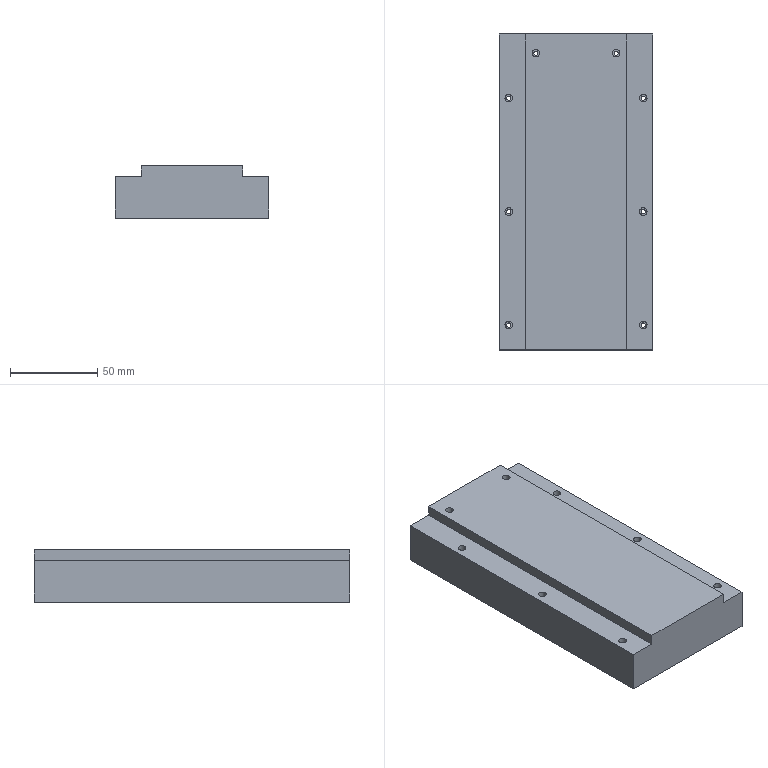Part | 2 solids | 364 faces | box 88 x 181.05 x 30 mm | volume 540458 mm3 | plane 181 | cylinder 121 | spline 40 | cone 22 | commonest cylinder face diameters 2.4 x24 4.4 x24 6 x17 1.6 x12 8 x7 1.161 x1